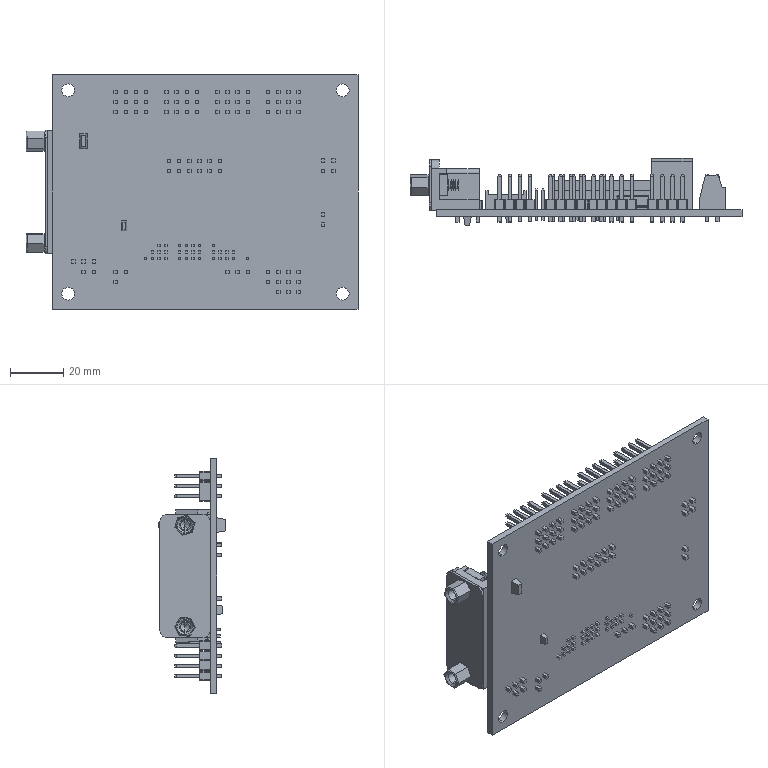Part | SolidWorks | features BaseBody 155, Scale 1 | 155 solids | 3002 faces | volume 58876 mm3 | plane 2861 | cylinder 87 | cone 48 | torus 6 | commonest cylinder face diameters 0.762 x30 2.857 x17 4.267 x12 3.391 x8 4.763 x8 5.334 x4